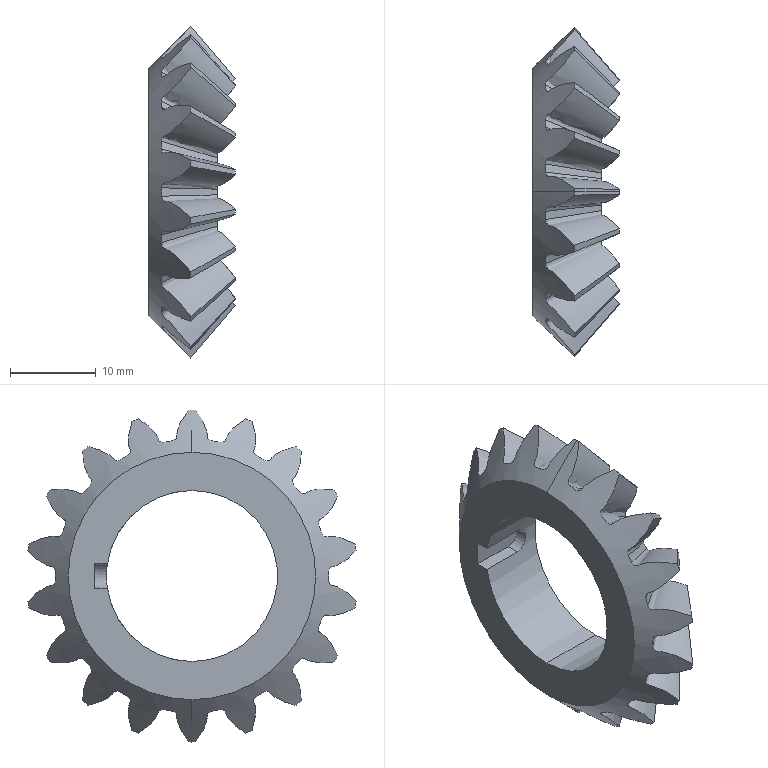Part | SolidWorks | features 3DProfileFeature 12, ICE 2, BlendCut 1, CirPattern 1, RefAxis 1, Revolution 1 | 1 solid | 102 faces | box 10.158 x 38.37 x 38.828 mm | volume 3651 mm3 | cone 40 | spline 36 | plane 23 | cylinder 3 | commonest cylinder face diameters 20 x2 3 x1